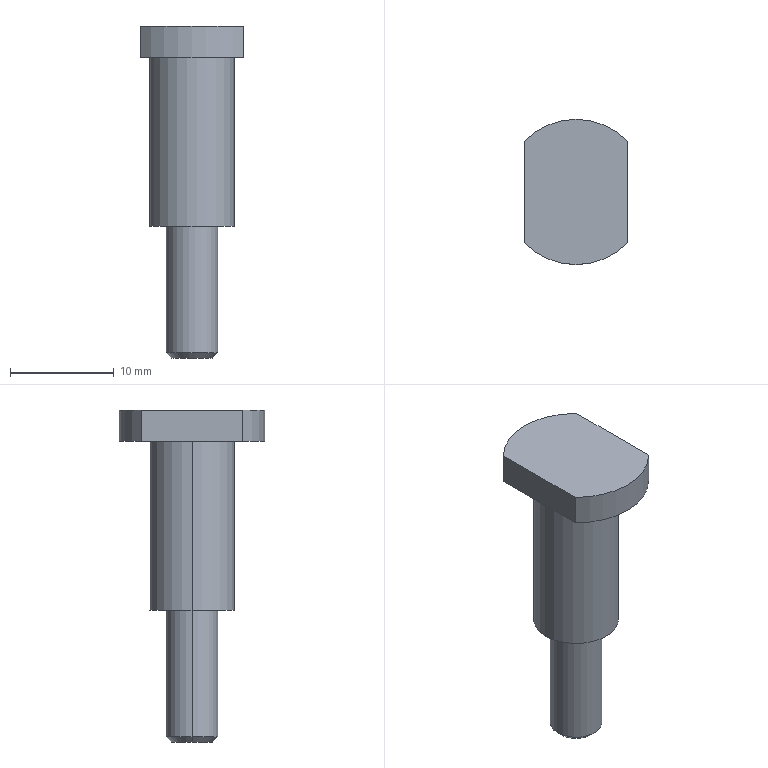Part | STEP file | 8XS900010 | 1 solid | 14 faces | box 10 x 14 x 32 mm | volume 1489 mm3 | cylinder 6 | plane 6 | cone 2 | commonest cylinder face diameters 5 x2 8.2 x2 14 x2
STEP:
#1=CARTESIAN_POINT('',(0.,0.,0.));
#2=DIRECTION('',(0.,0.,1.));
#3=DIRECTION('',(1.,0.,0.));
#4=AXIS2_PLACEMENT_3D('',#1,#2,#3);
#5=CARTESIAN_POINT('',(-2.,0.,-29.));
#6=VERTEX_POINT('',#5);
#7=CARTESIAN_POINT('',(2.,0.,-29.));
#8=VERTEX_POINT('',#7);
#9=CARTESIAN_POINT('',(0.,0.,-29.));
#10=DIRECTION('',(0.,0.,-1.));
#11=DIRECTION('',(-1.,0.,0.));
#12=AXIS2_PLACEMENT_3D('',#9,#10,#11);
#13=CIRCLE('',#12,2.);
#14=CARTESIAN_POINT('',(0.,0.,-29.));
#15=DIRECTION('',(0.,0.,1.));
#16=DIRECTION('',(1.,0.,0.));
#17=AXIS2_PLACEMENT_3D('',#14,#15,#16);
#18=CONICAL_SURFACE('',#17,2.,0.7854);
#19=CARTESIAN_POINT('',(3.142,0.));
#20=DIRECTION('',(-1.,0.));
#21=VECTOR('',#20,1.);
#22=LINE('',#19,#21);
#23=(GEOMETRIC_REPRESENTATION_CONTEXT(2)PARAMETRIC_REPRESENTATION_CONTEXT()REPRESENTATION_CONTEXT('',''));
#24=DEFINITIONAL_REPRESENTATION('',(#22),#23);
#25=PCURVE('',#18,#24);
#26=CARTESIAN_POINT('',(0.,0.,-29.));
#27=DIRECTION('',(0.,0.,-1.));
#28=DIRECTION('',(-1.,0.,0.));
#29=AXIS2_PLACEMENT_3D('',#26,#27,#28);
#30=PLANE('',#29);
#31=CARTESIAN_POINT('',(0.,0.));
#32=DIRECTION('',(1.,0.));
#33=AXIS2_PLACEMENT_2D('',#31,#32);
#34=CIRCLE('',#33,2.);
#35=(GEOMETRIC_REPRESENTATION_CONTEXT(2)PARAMETRIC_REPRESENTATION_CONTEXT()REPRESENTATION_CONTEXT('',''));
#36=DEFINITIONAL_REPRESENTATION('',(#34),#35);
#37=PCURVE('',#30,#36);
#38=SURFACE_CURVE('',#13,(#25,#37),.PCURVE_S1.);
#39=EDGE_CURVE('',#6,#8,#38,.T.);
#40=ORIENTED_EDGE('',*,*,#39,.F.);
#41=CARTESIAN_POINT('',(-2.5,0.,-28.5));
#42=VERTEX_POINT('',#41);
#43=CARTESIAN_POINT('',(-2.,0.,-29.));
#44=DIRECTION('',(-0.7071,0.,0.7071));
#45=VECTOR('',#44,1.);
#46=LINE('',#43,#45);
#47=CARTESIAN_POINT('',(3.142,0.));
#48=DIRECTION('',(0.,1.));
#49=VECTOR('',#48,1.);
#50=LINE('',#47,#49);
#51=(GEOMETRIC_REPRESENTATION_CONTEXT(2)PARAMETRIC_REPRESENTATION_CONTEXT()REPRESENTATION_CONTEXT('',''));
#52=DEFINITIONAL_REPRESENTATION('',(#50),#51);
#53=PCURVE('',#18,#52);
#54=CARTESIAN_POINT('',(0.,0.,-29.));
#55=DIRECTION('',(0.,0.,1.));
#56=DIRECTION('',(1.,0.,0.));
#57=AXIS2_PLACEMENT_3D('',#54,#55,#56);
#58=CONICAL_SURFACE('',#57,2.,0.7854);
#59=CARTESIAN_POINT('',(3.142,0.));
#60=DIRECTION('',(0.,1.));
#61=VECTOR('',#60,1.);
#62=LINE('',#59,#61);
#63=(GEOMETRIC_REPRESENTATION_CONTEXT(2)PARAMETRIC_REPRESENTATION_CONTEXT()REPRESENTATION_CONTEXT('',''));
#64=DEFINITIONAL_REPRESENTATION('',(#62),#63);
#65=PCURVE('',#58,#64);
#66=SURFACE_CURVE('',#46,(#53,#65),.PCURVE_S1.);
#67=EDGE_CURVE('',#6,#42,#66,.T.);
#68=ORIENTED_EDGE('',*,*,#67,.T.);
#69=CARTESIAN_POINT('',(2.5,0.,-28.5));
#70=VERTEX_POINT('',#69);
#71=CARTESIAN_POINT('',(0.,0.,-28.5));
#72=DIRECTION('',(0.,0.,1.));
#73=DIRECTION('',(-1.,0.,0.));
#74=AXIS2_PLACEMENT_3D('',#71,#72,#73);
#75=CIRCLE('',#74,2.5);
#76=CARTESIAN_POINT('',(-3.142,0.5));
#77=DIRECTION('',(1.,0.));
#78=VECTOR('',#77,1.);
#79=LINE('',#76,#78);
#80=(GEOMETRIC_REPRESENTATION_CONTEXT(2)PARAMETRIC_REPRESENTATION_CONTEXT()REPRESENTATION_CONTEXT('',''));
#81=DEFINITIONAL_REPRESENTATION('',(#79),#80);
#82=PCURVE('',#18,#81);
#83=CARTESIAN_POINT('',(0.,0.,-29.));
#84=DIRECTION('',(0.,0.,1.));
#85=DIRECTION('',(1.,0.,0.));
#86=AXIS2_PLACEMENT_3D('',#83,#84,#85);
#87=CYLINDRICAL_SURFACE('',#86,2.5);
#88=CARTESIAN_POINT('',(-3.142,0.5));
#89=DIRECTION('',(1.,0.));
#90=VECTOR('',#89,1.);
#91=LINE('',#88,#90);
#92=(GEOMETRIC_REPRESENTATION_CONTEXT(2)PARAMETRIC_REPRESENTATION_CONTEXT()REPRESENTATION_CONTEXT('',''));
#93=DEFINITIONAL_REPRESENTATION('',(#91),#92);
#94=PCURVE('',#87,#93);
#95=SURFACE_CURVE('',#75,(#82,#94),.PCURVE_S1.);
#96=EDGE_CURVE('',#70,#42,#95,.T.);
#97=ORIENTED_EDGE('',*,*,#96,.F.);
#98=CARTESIAN_POINT('',(2.,0.,-29.));
#99=DIRECTION('',(0.7071,0.,0.7071));
#100=VECTOR('',#99,1.);
#101=LINE('',#98,#100);
#102=CARTESIAN_POINT('',(0.,0.));
#103=DIRECTION('',(0.,1.));
#104=VECTOR('',#103,1.);
#105=LINE('',#102,#104);
#106=(GEOMETRIC_REPRESENTATION_CONTEXT(2)PARAMETRIC_REPRESENTATION_CONTEXT()REPRESENTATION_CONTEXT('',''));
#107=DEFINITIONAL_REPRESENTATION('',(#105),#106);
#108=PCURVE('',#18,#107);
#109=CARTESIAN_POINT('',(6.283,0.));
#110=DIRECTION('',(0.,1.));
#111=VECTOR('',#110,1.);
#112=LINE('',#109,#111);
#113=(GEOMETRIC_REPRESENTATION_CONTEXT(2)PARAMETRIC_REPRESENTATION_CONTEXT()REPRESENTATION_CONTEXT('',''));
#114=DEFINITIONAL_REPRESENTATION('',(#112),#113);
#115=PCURVE('',#58,#114);
#116=SURFACE_CURVE('',#101,(#108,#115),.PCURVE_S1.);
#117=EDGE_CURVE('',#8,#70,#116,.T.);
#118=ORIENTED_EDGE('',*,*,#117,.F.);
#119=EDGE_LOOP('',(#40,#68,#97,#118));
#120=FACE_BOUND('',#119,.T.);
#121=ADVANCED_FACE('',(#120),#18,.T.);
#122=ORIENTED_EDGE('',*,*,#96,.T.);
#123=CARTESIAN_POINT('',(-2.5,0.,-16.3));
#124=VERTEX_POINT('',#123);
#125=CARTESIAN_POINT('',(-2.5,0.,-29.));
#126=DIRECTION('',(0.,0.,1.));
#127=VECTOR('',#126,1.);
#128=LINE('',#125,#127);
#129=CARTESIAN_POINT('',(3.142,0.));
#130=DIRECTION('',(0.,1.));
#131=VECTOR('',#130,1.);
#132=LINE('',#129,#131);
#133=(GEOMETRIC_REPRESENTATION_CONTEXT(2)PARAMETRIC_REPRESENTATION_CONTEXT()REPRESENTATION_CONTEXT('',''));
#134=DEFINITIONAL_REPRESENTATION('',(#132),#133);
#135=PCURVE('',#87,#134);
#136=CARTESIAN_POINT('',(0.,0.,-29.));
#137=DIRECTION('',(0.,0.,1.));
#138=DIRECTION('',(1.,0.,0.));
#139=AXIS2_PLACEMENT_3D('',#136,#137,#138);
#140=CYLINDRICAL_SURFACE('',#139,2.5);
#141=CARTESIAN_POINT('',(3.142,0.));
#142=DIRECTION('',(0.,1.));
#143=VECTOR('',#142,1.);
#144=LINE('',#141,#143);
#145=(GEOMETRIC_REPRESENTATION_CONTEXT(2)PARAMETRIC_REPRESENTATION_CONTEXT()REPRESENTATION_CONTEXT('',''));
#146=DEFINITIONAL_REPRESENTATION('',(#144),#145);
#147=PCURVE('',#140,#146);
#148=SURFACE_CURVE('',#128,(#135,#147),.PCURVE_S1.);
#149=EDGE_CURVE('',#42,#124,#148,.T.);
#150=ORIENTED_EDGE('',*,*,#149,.T.);
#151=CARTESIAN_POINT('',(2.5,0.,-16.3));
#152=VERTEX_POINT('',#151);
#153=CARTESIAN_POINT('',(0.,0.,-16.3));
#154=DIRECTION('',(0.,0.,-1.));
#155=DIRECTION('',(-1.,0.,0.));
#156=AXIS2_PLACEMENT_3D('',#153,#154,#155);
#157=CIRCLE('',#156,2.5);
#158=CARTESIAN_POINT('',(3.142,12.7));
#159=DIRECTION('',(-1.,0.));
#160=VECTOR('',#159,1.);
#161=LINE('',#158,#160);
#162=(GEOMETRIC_REPRESENTATION_CONTEXT(2)PARAMETRIC_REPRESENTATION_CONTEXT()REPRESENTATION_CONTEXT('',''));
#163=DEFINITIONAL_REPRESENTATION('',(#161),#162);
#164=PCURVE('',#87,#163);
#165=CARTESIAN_POINT('',(0.,0.,-16.3));
#166=DIRECTION('',(0.,0.,-1.));
#167=DIRECTION('',(-1.,0.,0.));
#168=AXIS2_PLACEMENT_3D('',#165,#166,#167);
#169=PLANE('',#168);
#170=CARTESIAN_POINT('',(0.,0.));
#171=DIRECTION('',(1.,0.));
#172=AXIS2_PLACEMENT_2D('',#170,#171);
#173=CIRCLE('',#172,2.5);
#174=(GEOMETRIC_REPRESENTATION_CONTEXT(2)PARAMETRIC_REPRESENTATION_CONTEXT()REPRESENTATION_CONTEXT('',''));
#175=DEFINITIONAL_REPRESENTATION('',(#173),#174);
#176=PCURVE('',#169,#175);
#177=SURFACE_CURVE('',#157,(#164,#176),.PCURVE_S1.);
#178=EDGE_CURVE('',#124,#152,#177,.T.);
#179=ORIENTED_EDGE('',*,*,#178,.T.);
#180=CARTESIAN_POINT('',(2.5,0.,-29.));
#181=DIRECTION('',(0.,0.,1.));
#182=VECTOR('',#181,1.);
#183=LINE('',#180,#182);
#184=CARTESIAN_POINT('',(0.,0.));
#185=DIRECTION('',(0.,1.));
#186=VECTOR('',#185,1.);
#187=LINE('',#184,#186);
#188=(GEOMETRIC_REPRESENTATION_CONTEXT(2)PARAMETRIC_REPRESENTATION_CONTEXT()REPRESENTATION_CONTEXT('',''));
#189=DEFINITIONAL_REPRESENTATION('',(#187),#188);
#190=PCURVE('',#87,#189);
#191=CARTESIAN_POINT('',(6.283,0.));
#192=DIRECTION('',(0.,1.));
#193=VECTOR('',#192,1.);
#194=LINE('',#191,#193);
#195=(GEOMETRIC_REPRESENTATION_CONTEXT(2)PARAMETRIC_REPRESENTATION_CONTEXT()REPRESENTATION_CONTEXT('',''));
#196=DEFINITIONAL_REPRESENTATION('',(#194),#195);
#197=PCURVE('',#140,#196);
#198=SURFACE_CURVE('',#183,(#190,#197),.PCURVE_S1.);
#199=EDGE_CURVE('',#70,#152,#198,.T.);
#200=ORIENTED_EDGE('',*,*,#199,.F.);
#201=EDGE_LOOP('',(#122,#150,#179,#200));
#202=FACE_BOUND('',#201,.T.);
#203=ADVANCED_FACE('',(#202),#87,.T.);
#204=CARTESIAN_POINT('',(-4.1,0.,-16.3));
#205=VERTEX_POINT('',#204);
#206=CARTESIAN_POINT('',(4.1,0.,-16.3));
#207=VERTEX_POINT('',#206);
#208=CARTESIAN_POINT('',(0.,0.,-16.3));
#209=DIRECTION('',(0.,0.,-1.));
#210=DIRECTION('',(-1.,0.,0.));
#211=AXIS2_PLACEMENT_3D('',#208,#209,#210);
#212=CIRCLE('',#211,4.1);
#213=CARTESIAN_POINT('',(0.,0.,-16.3));
#214=DIRECTION('',(0.,0.,1.));
#215=DIRECTION('',(1.,0.,0.));
#216=AXIS2_PLACEMENT_3D('',#213,#214,#215);
#217=CYLINDRICAL_SURFACE('',#216,4.1);
#218=CARTESIAN_POINT('',(3.142,0.));
#219=DIRECTION('',(-1.,0.));
#220=VECTOR('',#219,1.);
#221=LINE('',#218,#220);
#222=(GEOMETRIC_REPRESENTATION_CONTEXT(2)PARAMETRIC_REPRESENTATION_CONTEXT()REPRESENTATION_CONTEXT('',''));
#223=DEFINITIONAL_REPRESENTATION('',(#221),#222);
#224=PCURVE('',#217,#223);
#225=CARTESIAN_POINT('',(0.,0.));
#226=DIRECTION('',(1.,0.));
#227=AXIS2_PLACEMENT_2D('',#225,#226);
#228=CIRCLE('',#227,4.1);
#229=(GEOMETRIC_REPRESENTATION_CONTEXT(2)PARAMETRIC_REPRESENTATION_CONTEXT()REPRESENTATION_CONTEXT('',''));
#230=DEFINITIONAL_REPRESENTATION('',(#228),#229);
#231=PCURVE('',#169,#230);
#232=SURFACE_CURVE('',#212,(#224,#231),.PCURVE_S1.);
#233=EDGE_CURVE('',#205,#207,#232,.T.);
#234=ORIENTED_EDGE('',*,*,#233,.F.);
#235=CARTESIAN_POINT('',(-4.1,0.,0.));
#236=VERTEX_POINT('',#235);
#237=CARTESIAN_POINT('',(-4.1,0.,-16.3));
#238=DIRECTION('',(0.,0.,1.));
#239=VECTOR('',#238,1.);
#240=LINE('',#237,#239);
#241=CARTESIAN_POINT('',(3.142,0.));
#242=DIRECTION('',(0.,1.));
#243=VECTOR('',#242,1.);
#244=LINE('',#241,#243);
#245=(GEOMETRIC_REPRESENTATION_CONTEXT(2)PARAMETRIC_REPRESENTATION_CONTEXT()REPRESENTATION_CONTEXT('',''));
#246=DEFINITIONAL_REPRESENTATION('',(#244),#245);
#247=PCURVE('',#217,#246);
#248=CARTESIAN_POINT('',(0.,0.,-16.3));
#249=DIRECTION('',(0.,0.,1.));
#250=DIRECTION('',(1.,0.,0.));
#251=AXIS2_PLACEMENT_3D('',#248,#249,#250);
#252=CYLINDRICAL_SURFACE('',#251,4.1);
#253=CARTESIAN_POINT('',(3.142,0.));
#254=DIRECTION('',(0.,1.));
#255=VECTOR('',#254,1.);
#256=LINE('',#253,#255);
#257=(GEOMETRIC_REPRESENTATION_CONTEXT(2)PARAMETRIC_REPRESENTATION_CONTEXT()REPRESENTATION_CONTEXT('',''));
#258=DEFINITIONAL_REPRESENTATION('',(#256),#257);
#259=PCURVE('',#252,#258);
#260=SURFACE_CURVE('',#240,(#247,#259),.PCURVE_S1.);
#261=EDGE_CURVE('',#205,#236,#260,.T.);
#262=ORIENTED_EDGE('',*,*,#261,.T.);
#263=CARTESIAN_POINT('',(4.1,0.,0.));
#264=VERTEX_POINT('',#263);
#265=CARTESIAN_POINT('',(0.,0.,0.));
#266=DIRECTION('',(0.,0.,-1.));
#267=DIRECTION('',(1.,0.,0.));
#268=AXIS2_PLACEMENT_3D('',#265,#266,#267);
#269=CIRCLE('',#268,4.1);
#270=CARTESIAN_POINT('',(6.283,16.3));
#271=DIRECTION('',(-1.,0.));
#272=VECTOR('',#271,1.);
#273=LINE('',#270,#272);
#274=(GEOMETRIC_REPRESENTATION_CONTEXT(2)PARAMETRIC_REPRESENTATION_CONTEXT()REPRESENTATION_CONTEXT('',''));
#275=DEFINITIONAL_REPRESENTATION('',(#273),#274);
#276=PCURVE('',#217,#275);
#277=CARTESIAN_POINT('',(0.,0.,0.));
#278=DIRECTION('',(0.,0.,1.));
#279=DIRECTION('',(1.,0.,0.));
#280=AXIS2_PLACEMENT_3D('',#277,#278,#279);
#281=PLANE('',#280);
#282=CARTESIAN_POINT('',(4.1,0.));
#283=CARTESIAN_POINT('',(4.1,-7.101));
#284=CARTESIAN_POINT('',(-2.05,-3.551));
#285=CARTESIAN_POINT('',(-8.2,0.));
#286=CARTESIAN_POINT('',(-2.05,3.551));
#287=CARTESIAN_POINT('',(4.1,7.101));
#288=CARTESIAN_POINT('',(4.1,0.));
#289=(BOUNDED_CURVE()B_SPLINE_CURVE(2,(#282,#283,#284,#285,#286,#287,#288),.UNSPECIFIED.,.T.,.F.)B_SPLINE_CURVE_WITH_KNOTS((1,2,2,2,2,1),(-2.094,0.,2.094,4.189,6.283,8.378),.UNSPECIFIED.)CURVE()GEOMETRIC_REPRESENTATION_ITEM()RATIONAL_B_SPLINE_CURVE((1.,0.5,1.,0.5,1.,0.5,1.))REPRESENTATION_ITEM(''));
#290=(GEOMETRIC_REPRESENTATION_CONTEXT(2)PARAMETRIC_REPRESENTATION_CONTEXT()REPRESENTATION_CONTEXT('',''));
#291=DEFINITIONAL_REPRESENTATION('',(#289),#290);
#292=PCURVE('',#281,#291);
#293=SURFACE_CURVE('',#269,(#276,#292),.PCURVE_S1.);
#294=EDGE_CURVE('',#236,#264,#293,.T.);
#295=ORIENTED_EDGE('',*,*,#294,.T.);
#296=CARTESIAN_POINT('',(4.1,0.,-16.3));
#297=DIRECTION('',(0.,0.,1.));
#298=VECTOR('',#297,1.);
#299=LINE('',#296,#298);
#300=CARTESIAN_POINT('',(0.,0.));
#301=DIRECTION('',(0.,1.));
#302=VECTOR('',#301,1.);
#303=LINE('',#300,#302);
#304=(GEOMETRIC_REPRESENTATION_CONTEXT(2)PARAMETRIC_REPRESENTATION_CONTEXT()REPRESENTATION_CONTEXT('',''));
#305=DEFINITIONAL_REPRESENTATION('',(#303),#304);
#306=PCURVE('',#217,#305);
#307=CARTESIAN_POINT('',(6.283,0.));
#308=DIRECTION('',(0.,1.));
#309=VECTOR('',#308,1.);
#310=LINE('',#307,#309);
#311=(GEOMETRIC_REPRESENTATION_CONTEXT(2)PARAMETRIC_REPRESENTATION_CONTEXT()REPRESENTATION_CONTEXT('',''));
#312=DEFINITIONAL_REPRESENTATION('',(#310),#311);
#313=PCURVE('',#252,#312);
#314=SURFACE_CURVE('',#299,(#306,#313),.PCURVE_S1.);
#315=EDGE_CURVE('',#207,#264,#314,.T.);
#316=ORIENTED_EDGE('',*,*,#315,.F.);
#317=EDGE_LOOP('',(#234,#262,#295,#316));
#318=FACE_BOUND('',#317,.T.);
#319=ADVANCED_FACE('',(#318),#217,.T.);
#320=CARTESIAN_POINT('',(0.,0.,-16.3));
#321=DIRECTION('',(0.,0.,-1.));
#322=DIRECTION('',(-1.,0.,0.));
#323=AXIS2_PLACEMENT_3D('',#320,#321,#322);
#324=CIRCLE('',#323,4.1);
#325=CARTESIAN_POINT('',(0.,0.));
#326=DIRECTION('',(1.,0.));
#327=AXIS2_PLACEMENT_2D('',#325,#326);
#328=CIRCLE('',#327,4.1);
#329=(GEOMETRIC_REPRESENTATION_CONTEXT(2)PARAMETRIC_REPRESENTATION_CONTEXT()REPRESENTATION_CONTEXT('',''));
#330=DEFINITIONAL_REPRESENTATION('',(#328),#329);
#331=PCURVE('',#169,#330);
#332=CARTESIAN_POINT('',(9.425,0.));
#333=DIRECTION('',(-1.,0.));
#334=VECTOR('',#333,1.);
#335=LINE('',#332,#334);
#336=(GEOMETRIC_REPRESENTATION_CONTEXT(2)PARAMETRIC_REPRESENTATION_CONTEXT()REPRESENTATION_CONTEXT('',''));
#337=DEFINITIONAL_REPRESENTATION('',(#335),#336);
#338=PCURVE('',#252,#337);
#339=SURFACE_CURVE('',#324,(#331,#338),.PCURVE_S1.);
#340=EDGE_CURVE('',#207,#205,#339,.T.);
#341=ORIENTED_EDGE('',*,*,#340,.T.);
#342=ORIENTED_EDGE('',*,*,#233,.T.);
#343=EDGE_LOOP('',(#341,#342));
#344=FACE_BOUND('',#343,.T.);
#345=CARTESIAN_POINT('',(0.,0.,-16.3));
#346=DIRECTION('',(0.,0.,-1.));
#347=DIRECTION('',(-1.,0.,0.));
#348=AXIS2_PLACEMENT_3D('',#345,#346,#347);
#349=CIRCLE('',#348,2.5);
#350=CARTESIAN_POINT('',(0.,0.));
#351=DIRECTION('',(1.,0.));
#352=AXIS2_PLACEMENT_2D('',#350,#351);
#353=CIRCLE('',#352,2.5);
#354=(GEOMETRIC_REPRESENTATION_CONTEXT(2)PARAMETRIC_REPRESENTATION_CONTEXT()REPRESENTATION_CONTEXT('',''));
#355=DEFINITIONAL_REPRESENTATION('',(#353),#354);
#356=PCURVE('',#169,#355);
#357=CARTESIAN_POINT('',(9.425,12.7));
#358=DIRECTION('',(-1.,0.));
#359=VECTOR('',#358,1.);
#360=LINE('',#357,#359);
#361=(GEOMETRIC_REPRESENTATION_CONTEXT(2)PARAMETRIC_REPRESENTATION_CONTEXT()REPRESENTATION_CONTEXT('',''));
#362=DEFINITIONAL_REPRESENTATION('',(#360),#361);
#363=PCURVE('',#140,#362);
#364=SURFACE_CURVE('',#349,(#356,#363),.PCURVE_S1.);
#365=EDGE_CURVE('',#152,#124,#364,.T.);
#366=ORIENTED_EDGE('',*,*,#365,.F.);
#367=ORIENTED_EDGE('',*,*,#178,.F.);
#368=EDGE_LOOP('',(#366,#367));
#369=FACE_BOUND('',#368,.T.);
#370=ADVANCED_FACE('',(#344,#369),#169,.T.);
#371=CARTESIAN_POINT('',(5.,4.899,0.));
#372=VERTEX_POINT('',#371);
#373=CARTESIAN_POINT('',(-5.,4.899,0.));
#374=VERTEX_POINT('',#373);
#375=CARTESIAN_POINT('',(0.,0.,0.));
#376=DIRECTION('',(0.,0.,1.));
#377=DIRECTION('',(1.,0.,0.));
#378=AXIS2_PLACEMENT_3D('',#375,#376,#377);
#379=CIRCLE('',#378,7.);
#380=CARTESIAN_POINT('',(0.,0.));
#381=DIRECTION('',(1.,0.));
#382=AXIS2_PLACEMENT_2D('',#380,#381);
#383=CIRCLE('',#382,7.);
#384=(GEOMETRIC_REPRESENTATION_CONTEXT(2)PARAMETRIC_REPRESENTATION_CONTEXT()REPRESENTATION_CONTEXT('',''));
#385=DEFINITIONAL_REPRESENTATION('',(#383),#384);
#386=PCURVE('',#281,#385);
#387=CARTESIAN_POINT('',(0.,0.,3.));
#388=DIRECTION('',(0.,0.,-1.));
#389=DIRECTION('',(-1.,0.,0.));
#390=AXIS2_PLACEMENT_3D('',#387,#388,#389);
#391=CYLINDRICAL_SURFACE('',#390,7.);
#392=CARTESIAN_POINT('',(3.142,3.));
#393=DIRECTION('',(-1.,0.));
#394=VECTOR('',#393,1.);
#395=LINE('',#392,#394);
#396=(GEOMETRIC_REPRESENTATION_CONTEXT(2)PARAMETRIC_REPRESENTATION_CONTEXT()REPRESENTATION_CONTEXT('',''));
#397=DEFINITIONAL_REPRESENTATION('',(#395),#396);
#398=PCURVE('',#391,#397);
#399=SURFACE_CURVE('',#379,(#386,#398),.PCURVE_S1.);
#400=EDGE_CURVE('',#372,#374,#399,.T.);
#401=ORIENTED_EDGE('',*,*,#400,.F.);
#402=CARTESIAN_POINT('',(5.,-4.899,0.));
#403=VERTEX_POINT('',#402);
#404=CARTESIAN_POINT('',(5.,4.899,0.));
#405=DIRECTION('',(0.,1.,0.));
#406=VECTOR('',#405,1.);
#407=LINE('',#404,#406);
#408=CARTESIAN_POINT('',(5.,4.899));
#409=DIRECTION('',(0.,1.));
#410=VECTOR('',#409,1.);
#411=LINE('',#408,#410);
#412=(GEOMETRIC_REPRESENTATION_CONTEXT(2)PARAMETRIC_REPRESENTATION_CONTEXT()REPRESENTATION_CONTEXT('',''));
#413=DEFINITIONAL_REPRESENTATION('',(#411),#412);
#414=PCURVE('',#281,#413);
#415=CARTESIAN_POINT('',(5.,4.899,3.));
#416=DIRECTION('',(-1.,0.,0.));
#417=DIRECTION('',(0.,0.,1.));
#418=AXIS2_PLACEMENT_3D('',#415,#416,#417);
#419=PLANE('',#418);
#420=CARTESIAN_POINT('',(-3.,0.));
#421=DIRECTION('',(0.,1.));
#422=VECTOR('',#421,1.);
#423=LINE('',#420,#422);
#424=(GEOMETRIC_REPRESENTATION_CONTEXT(2)PARAMETRIC_REPRESENTATION_CONTEXT()REPRESENTATION_CONTEXT('',''));
#425=DEFINITIONAL_REPRESENTATION('',(#423),#424);
#426=PCURVE('',#419,#425);
#427=SURFACE_CURVE('',#407,(#414,#426),.PCURVE_S1.);
#428=EDGE_CURVE('',#403,#372,#427,.T.);
#429=ORIENTED_EDGE('',*,*,#428,.F.);
#430=CARTESIAN_POINT('',(-5.,-4.899,0.));
#431=VERTEX_POINT('',#430);
#432=CARTESIAN_POINT('',(0.,0.,0.));
#433=DIRECTION('',(0.,0.,1.));
#434=DIRECTION('',(1.,0.,0.));
#435=AXIS2_PLACEMENT_3D('',#432,#433,#434);
#436=CIRCLE('',#435,7.);
#437=CARTESIAN_POINT('',(0.,0.));
#438=DIRECTION('',(1.,0.));
#439=AXIS2_PLACEMENT_2D('',#437,#438);
#440=CIRCLE('',#439,7.);
#441=(GEOMETRIC_REPRESENTATION_CONTEXT(2)PARAMETRIC_REPRESENTATION_CONTEXT()REPRESENTATION_CONTEXT('',''));
#442=DEFINITIONAL_REPRESENTATION('',(#440),#441);
#443=PCURVE('',#281,#442);
#444=CARTESIAN_POINT('',(0.,0.,3.));
#445=DIRECTION('',(0.,0.,-1.));
#446=DIRECTION('',(-1.,0.,0.));
#447=AXIS2_PLACEMENT_3D('',#444,#445,#446);
#448=CYLINDRICAL_SURFACE('',#447,7.);
#449=CARTESIAN_POINT('',(9.425,3.));
#450=DIRECTION('',(-1.,0.));
#451=VECTOR('',#450,1.);
#452=LINE('',#449,#451);
#453=(GEOMETRIC_REPRESENTATION_CONTEXT(2)PARAMETRIC_REPRESENTATION_CONTEXT()REPRESENTATION_CONTEXT('',''));
#454=DEFINITIONAL_REPRESENTATION('',(#452),#453);
#455=PCURVE('',#448,#454);
#456=SURFACE_CURVE('',#436,(#443,#455),.PCURVE_S1.);
#457=EDGE_CURVE('',#431,#403,#456,.T.);
#458=ORIENTED_EDGE('',*,*,#457,.F.);
#459=CARTESIAN_POINT('',(-5.,4.899,0.));
#460=DIRECTION('',(0.,-1.,0.));
#461=VECTOR('',#460,1.);
#462=LINE('',#459,#461);
#463=CARTESIAN_POINT('',(-5.,4.899));
#464=DIRECTION('',(0.,-1.));
#465=VECTOR('',#464,1.);
#466=LINE('',#463,#465);
#467=(GEOMETRIC_REPRESENTATION_CONTEXT(2)PARAMETRIC_REPRESENTATION_CONTEXT()REPRESENTATION_CONTEXT('',''));
#468=DEFINITIONAL_REPRESENTATION('',(#466),#467);
#469=PCURVE('',#281,#468);
#470=CARTESIAN_POINT('',(-5.,4.899,3.));
#471=DIRECTION('',(1.,0.,0.));
#472=DIRECTION('',(0.,0.,-1.));
#473=AXIS2_PLACEMENT_3D('',#470,#471,#472);
#474=PLANE('',#473);
#475=CARTESIAN_POINT('',(3.,0.));
#476=DIRECTION('',(0.,-1.));
#477=VECTOR('',#476,1.);
#478=LINE('',#475,#477);
#479=(GEOMETRIC_REPRESENTATION_CONTEXT(2)PARAMETRIC_REPRESENTATION_CONTEXT()REPRESENTATION_CONTEXT('',''));
#480=DEFINITIONAL_REPRESENTATION('',(#478),#479);
#481=PCURVE('',#474,#480);
#482=SURFACE_CURVE('',#462,(#469,#481),.PCURVE_S1.);
#483=EDGE_CURVE('',#374,#431,#482,.T.);
#484=ORIENTED_EDGE('',*,*,#483,.F.);
#485=EDGE_LOOP('',(#401,#429,#458,#484));
#486=FACE_BOUND('',#485,.T.);
#487=CARTESIAN_POINT('',(0.,0.,0.));
#488=DIRECTION('',(0.,0.,-1.));
#489=DIRECTION('',(1.,0.,0.));
#490=AXIS2_PLACEMENT_3D('',#487,#488,#489);
#491=CIRCLE('',#490,4.1);
#492=CARTESIAN_POINT('',(4.1,0.));
#493=CARTESIAN_POINT('',(4.1,-7.101));
#494=CARTESIAN_POINT('',(-2.05,-3.551));
#495=CARTESIAN_POINT('',(-8.2,0.));
#496=CARTESIAN_POINT('',(-2.05,3.551));
#497=CARTESIAN_POINT('',(4.1,7.101));
#498=CARTESIAN_POINT('',(4.1,0.));
#499=(BOUNDED_CURVE()B_SPLINE_CURVE(2,(#492,#493,#494,#495,#496,#497,#498),.UNSPECIFIED.,.T.,.F.)B_SPLINE_CURVE_WITH_KNOTS((1,2,2,2,2,1),(-2.094,0.,2.094,4.189,6.283,8.378),.UNSPECIFIED.)CURVE()GEOMETRIC_REPRESENTATION_ITEM()RATIONAL_B_SPLINE_CURVE((1.,0.5,1.,0.5,1.,0.5,1.))REPRESENTATION_ITEM(''));
#500=(GEOMETRIC_REPRESENTATION_CONTEXT(2)PARAMETRIC_REPRESENTATION_CONTEXT()REPRESENTATION_CONTEXT('',''));
#501=DEFINITIONAL_REPRESENTATION('',(#499),#500);
#502=PCURVE('',#281,#501);
#503=CARTESIAN_POINT('',(6.283,16.3));
#504=DIRECTION('',(-1.,0.));
#505=VECTOR('',#504,1.);
#506=LINE('',#503,#505);
#507=(GEOMETRIC_REPRESENTATION_CONTEXT(2)PARAMETRIC_REPRESENTATION_CONTEXT()REPRESENTATION_CONTEXT('',''));
#508=DEFINITIONAL_REPRESENTATION('',(#506),#507);
#509=PCURVE('',#252,#508);
#510=SURFACE_CURVE('',#491,(#502,#509),.PCURVE_S1.);
#511=EDGE_CURVE('',#264,#236,#510,.T.);
#512=ORIENTED_EDGE('',*,*,#511,.F.);
#513=ORIENTED_EDGE('',*,*,#294,.F.);
#514=EDGE_LOOP('',(#512,#513));
#515=FACE_BOUND('',#514,.T.);
#516=ADVANCED_FACE('',(#486,#515),#281,.F.);
#517=ORIENTED_EDGE('',*,*,#400,.T.);
#518=CARTESIAN_POINT('',(-5.,4.899,3.));
#519=VERTEX_POINT('',#518);
#520=CARTESIAN_POINT('',(-5.,4.899,3.));
#521=DIRECTION('',(0.,0.,-1.));
#522=VECTOR('',#521,1.);
#523=LINE('',#520,#522);
#524=CARTESIAN_POINT('',(0.7752,0.));
#525=DIRECTION('',(0.,1.));
#526=VECTOR('',#525,1.);
#527=LINE('',#524,#526);
#528=(GEOMETRIC_REPRESENTATION_CONTEXT(2)PARAMETRIC_REPRESENTATION_CONTEXT()REPRESENTATION_CONTEXT('',''));
#529=DEFINITIONAL_REPRESENTATION('',(#527),#528);
#530=PCURVE('',#391,#529);
#531=CARTESIAN_POINT('',(0.,0.));
#532=DIRECTION('',(1.,0.));
#533=VECTOR('',#532,1.);
#534=LINE('',#531,#533);
#535=(GEOMETRIC_REPRESENTATION_CONTEXT(2)PARAMETRIC_REPRESENTATION_CONTEXT()REPRESENTATION_CONTEXT('',''));
#536=DEFINITIONAL_REPRESENTATION('',(#534),#535);
#537=PCURVE('',#474,#536);
#538=SURFACE_CURVE('',#523,(#530,#537),.PCURVE_S1.);
#539=EDGE_CURVE('',#519,#374,#538,.T.);
#540=ORIENTED_EDGE('',*,*,#539,.F.);
#541=CARTESIAN_POINT('',(5.,4.899,3.));
#542=VERTEX_POINT('',#541);
#543=CARTESIAN_POINT('',(0.,0.,3.));
#544=DIRECTION('',(0.,0.,1.));
#545=DIRECTION('',(1.,0.,0.));
#546=AXIS2_PLACEMENT_3D('',#543,#544,#545);
#547=CIRCLE('',#546,7.);
#548=CARTESIAN_POINT('',(3.142,0.));
#549=DIRECTION('',(-1.,0.));
#550=VECTOR('',#549,1.);
#551=LINE('',#548,#550);
#552=(GEOMETRIC_REPRESENTATION_CONTEXT(2)PARAMETRIC_REPRESENTATION_CONTEXT()REPRESENTATION_CONTEXT('',''));
#553=DEFINITIONAL_REPRESENTATION('',(#551),#552);
#554=PCURVE('',#391,#553);
#555=CARTESIAN_POINT('',(0.,0.,3.));
#556=DIRECTION('',(0.,0.,1.));
#557=DIRECTION('',(1.,0.,0.));
#558=AXIS2_PLACEMENT_3D('',#555,#556,#557);
#559=PLANE('',#558);
#560=CARTESIAN_POINT('',(0.,0.));
#561=DIRECTION('',(1.,0.));
#562=AXIS2_PLACEMENT_2D('',#560,#561);
#563=CIRCLE('',#562,7.);
#564=(GEOMETRIC_REPRESENTATION_CONTEXT(2)PARAMETRIC_REPRESENTATION_CONTEXT()REPRESENTATION_CONTEXT('',''));
#565=DEFINITIONAL_REPRESENTATION('',(#563),#564);
#566=PCURVE('',#559,#565);
#567=SURFACE_CURVE('',#547,(#554,#566),.PCURVE_S1.);
#568=EDGE_CURVE('',#542,#519,#567,.T.);
#569=ORIENTED_EDGE('',*,*,#568,.F.);
#570=CARTESIAN_POINT('',(5.,4.899,3.));
#571=DIRECTION('',(0.,0.,-1.));
#572=VECTOR('',#571,1.);
#573=LINE('',#570,#572);
#574=CARTESIAN_POINT('',(2.366,0.));
#575=DIRECTION('',(0.,1.));
#576=VECTOR('',#575,1.);
#577=LINE('',#574,#576);
#578=(GEOMETRIC_REPRESENTATION_CONTEXT(2)PARAMETRIC_REPRESENTATION_CONTEXT()REPRESENTATION_CONTEXT('',''));
#579=DEFINITIONAL_REPRESENTATION('',(#577),#578);
#580=PCURVE('',#391,#579);
#581=CARTESIAN_POINT('',(0.,0.));
#582=DIRECTION('',(-1.,0.));
#583=VECTOR('',#582,1.);
#584=LINE('',#581,#583);
#585=(GEOMETRIC_REPRESENTATION_CONTEXT(2)PARAMETRIC_REPRESENTATION_CONTEXT()REPRESENTATION_CONTEXT('',''));
#586=DEFINITIONAL_REPRESENTATION('',(#584),#585);
#587=PCURVE('',#419,#586);
#588=SURFACE_CURVE('',#573,(#580,#587),.PCURVE_S1.);
#589=EDGE_CURVE('',#542,#372,#588,.T.);
#590=ORIENTED_EDGE('',*,*,#589,.T.);
#591=EDGE_LOOP('',(#517,#540,#569,#590));
#592=FACE_BOUND('',#591,.T.);
#593=ADVANCED_FACE('',(#592),#391,.T.);
#594=ORIENTED_EDGE('',*,*,#483,.T.);
#595=CARTESIAN_POINT('',(-5.,-4.899,3.));
#596=VERTEX_POINT('',#595);
#597=CARTESIAN_POINT('',(-5.,-4.899,3.));
#598=DIRECTION('',(0.,0.,-1.));
#599=VECTOR('',#598,1.);
#600=LINE('',#597,#599);
#601=CARTESIAN_POINT('',(0.,-9.798));
#602=DIRECTION('',(1.,0.));
#603=VECTOR('',#602,1.);
#604=LINE('',#601,#603);
#605=(GEOMETRIC_REPRESENTATION_CONTEXT(2)PARAMETRIC_REPRESENTATION_CONTEXT()REPRESENTATION_CONTEXT('',''));
#606=DEFINITIONAL_REPRESENTATION('',(#604),#605);
#607=PCURVE('',#474,#606);
#608=CARTESIAN_POINT('',(5.508,0.));
#609=DIRECTION('',(0.,1.));
#610=VECTOR('',#609,1.);
#611=LINE('',#608,#610);
#612=(GEOMETRIC_REPRESENTATION_CONTEXT(2)PARAMETRIC_REPRESENTATION_CONTEXT()REPRESENTATION_CONTEXT('',''));
#613=DEFINITIONAL_REPRESENTATION('',(#611),#612);
#614=PCURVE('',#448,#613);
#615=SURFACE_CURVE('',#600,(#607,#614),.PCURVE_S1.);
#616=EDGE_CURVE('',#596,#431,#615,.T.);
#617=ORIENTED_EDGE('',*,*,#616,.F.);
#618=CARTESIAN_POINT('',(-5.,4.899,3.));
#619=DIRECTION('',(0.,-1.,0.));
#620=VECTOR('',#619,1.);
#621=LINE('',#618,#620);
#622=CARTESIAN_POINT('',(0.,0.));
#623=DIRECTION('',(0.,-1.));
#624=VECTOR('',#623,1.);
#625=LINE('',#622,#624);
#626=(GEOMETRIC_REPRESENTATION_CONTEXT(2)PARAMETRIC_REPRESENTATION_CONTEXT()REPRESENTATION_CONTEXT('',''));
#627=DEFINITIONAL_REPRESENTATION('',(#625),#626);
#628=PCURVE('',#474,#627);
#629=CARTESIAN_POINT('',(-5.,4.899));
#630=DIRECTION('',(0.,-1.));
#631=VECTOR('',#630,1.);
#632=LINE('',#629,#631);
#633=(GEOMETRIC_REPRESENTATION_CONTEXT(2)PARAMETRIC_REPRESENTATION_CONTEXT()REPRESENTATION_CONTEXT('',''));
#634=DEFINITIONAL_REPRESENTATION('',(#632),#633);
#635=PCURVE('',#559,#634);
#636=SURFACE_CURVE('',#621,(#628,#635),.PCURVE_S1.);
#637=EDGE_CURVE('',#519,#596,#636,.T.);
#638=ORIENTED_EDGE('',*,*,#637,.F.);
#639=ORIENTED_EDGE('',*,*,#539,.T.);
#640=EDGE_LOOP('',(#594,#617,#638,#639));
#641=FACE_BOUND('',#640,.T.);
#642=ADVANCED_FACE('',(#641),#474,.F.);
#643=ORIENTED_EDGE('',*,*,#457,.T.);
#644=CARTESIAN_POINT('',(5.,-4.899,3.));
#645=VERTEX_POINT('',#644);
#646=CARTESIAN_POINT('',(5.,-4.899,3.));
#647=DIRECTION('',(0.,0.,-1.));
#648=VECTOR('',#647,1.);
#649=LINE('',#646,#648);
#650=CARTESIAN_POINT('',(3.917,0.));
#651=DIRECTION('',(0.,1.));
#652=VECTOR('',#651,1.);
#653=LINE('',#650,#652);
#654=(GEOMETRIC_REPRESENTATION_CONTEXT(2)PARAMETRIC_REPRESENTATION_CONTEXT()REPRESENTATION_CONTEXT('',''));
#655=DEFINITIONAL_REPRESENTATION('',(#653),#654);
#656=PCURVE('',#448,#655);
#657=CARTESIAN_POINT('',(0.,-9.798));
#658=DIRECTION('',(-1.,0.));
#659=VECTOR('',#658,1.);
#660=LINE('',#657,#659);
#661=(GEOMETRIC_REPRESENTATION_CONTEXT(2)PARAMETRIC_REPRESENTATION_CONTEXT()REPRESENTATION_CONTEXT('',''));
#662=DEFINITIONAL_REPRESENTATION('',(#660),#661);
#663=PCURVE('',#419,#662);
#664=SURFACE_CURVE('',#649,(#656,#663),.PCURVE_S1.);
#665=EDGE_CURVE('',#645,#403,#664,.T.);
#666=ORIENTED_EDGE('',*,*,#665,.F.);
#667=CARTESIAN_POINT('',(0.,0.,3.));
#668=DIRECTION('',(0.,0.,1.));
#669=DIRECTION('',(1.,0.,0.));
#670=AXIS2_PLACEMENT_3D('',#667,#668,#669);
#671=CIRCLE('',#670,7.);
#672=CARTESIAN_POINT('',(9.425,0.));
#673=DIRECTION('',(-1.,0.));
#674=VECTOR('',#673,1.);
#675=LINE('',#672,#674);
#676=(GEOMETRIC_REPRESENTATION_CONTEXT(2)PARAMETRIC_REPRESENTATION_CONTEXT()REPRESENTATION_CONTEXT('',''));
#677=DEFINITIONAL_REPRESENTATION('',(#675),#676);
#678=PCURVE('',#448,#677);
#679=CARTESIAN_POINT('',(0.,0.));
#680=DIRECTION('',(1.,0.));
#681=AXIS2_PLACEMENT_2D('',#679,#680);
#682=CIRCLE('',#681,7.);
#683=(GEOMETRIC_REPRESENTATION_CONTEXT(2)PARAMETRIC_REPRESENTATION_CONTEXT()REPRESENTATION_CONTEXT('',''));
#684=DEFINITIONAL_REPRESENTATION('',(#682),#683);
#685=PCURVE('',#559,#684);
#686=SURFACE_CURVE('',#671,(#678,#685),.PCURVE_S1.);
#687=EDGE_CURVE('',#596,#645,#686,.T.);
#688=ORIENTED_EDGE('',*,*,#687,.F.);
#689=ORIENTED_EDGE('',*,*,#616,.T.);
#690=EDGE_LOOP('',(#643,#666,#688,#689));
#691=FACE_BOUND('',#690,.T.);
#692=ADVANCED_FACE('',(#691),#448,.T.);
#693=ORIENTED_EDGE('',*,*,#428,.T.);
#694=ORIENTED_EDGE('',*,*,#589,.F.);
#695=CARTESIAN_POINT('',(5.,4.899,3.));
#696=DIRECTION('',(0.,1.,0.));
#697=VECTOR('',#696,1.);
#698=LINE('',#695,#697);
#699=CARTESIAN_POINT('',(0.,0.));
#700=DIRECTION('',(0.,1.));
#701=VECTOR('',#700,1.);
#702=LINE('',#699,#701);
#703=(GEOMETRIC_REPRESENTATION_CONTEXT(2)PARAMETRIC_REPRESENTATION_CONTEXT()REPRESENTATION_CONTEXT('',''));
#704=DEFINITIONAL_REPRESENTATION('',(#702),#703);
#705=PCURVE('',#419,#704);
#706=CARTESIAN_POINT('',(5.,4.899));
#707=DIRECTION('',(0.,1.));
#708=VECTOR('',#707,1.);
#709=LINE('',#706,#708);
#710=(GEOMETRIC_REPRESENTATION_CONTEXT(2)PARAMETRIC_REPRESENTATION_CONTEXT()REPRESENTATION_CONTEXT('',''));
#711=DEFINITIONAL_REPRESENTATION('',(#709),#710);
#712=PCURVE('',#559,#711);
#713=SURFACE_CURVE('',#698,(#705,#712),.PCURVE_S1.);
#714=EDGE_CURVE('',#645,#542,#713,.T.);
#715=ORIENTED_EDGE('',*,*,#714,.F.);
#716=ORIENTED_EDGE('',*,*,#665,.T.);
#717=EDGE_LOOP('',(#693,#694,#715,#716));
#718=FACE_BOUND('',#717,.T.);
#719=ADVANCED_FACE('',(#718),#419,.F.);
#720=ORIENTED_EDGE('',*,*,#568,.T.);
#721=ORIENTED_EDGE('',*,*,#637,.T.);
#722=ORIENTED_EDGE('',*,*,#687,.T.);
#723=ORIENTED_EDGE('',*,*,#714,.T.);
#724=EDGE_LOOP('',(#720,#721,#722,#723));
#725=FACE_BOUND('',#724,.T.);
#726=ADVANCED_FACE('',(#725),#559,.T.);
#727=ORIENTED_EDGE('',*,*,#261,.F.);
#728=ORIENTED_EDGE('',*,*,#340,.F.);
#729=ORIENTED_EDGE('',*,*,#315,.T.);
#730=ORIENTED_EDGE('',*,*,#511,.T.);
#731=EDGE_LOOP('',(#727,#728,#729,#730));
#732=FACE_BOUND('',#731,.T.);
#733=ADVANCED_FACE('',(#732),#252,.T.);
#734=ORIENTED_EDGE('',*,*,#149,.F.);
#735=CARTESIAN_POINT('',(0.,0.,-28.5));
#736=DIRECTION('',(0.,0.,1.));
#737=DIRECTION('',(-1.,0.,0.));
#738=AXIS2_PLACEMENT_3D('',#735,#736,#737);
#739=CIRCLE('',#738,2.5);
#740=CARTESIAN_POINT('',(3.142,0.5));
#741=DIRECTION('',(1.,0.));
#742=VECTOR('',#741,1.);
#743=LINE('',#740,#742);
#744=(GEOMETRIC_REPRESENTATION_CONTEXT(2)PARAMETRIC_REPRESENTATION_CONTEXT()REPRESENTATION_CONTEXT('',''));
#745=DEFINITIONAL_REPRESENTATION('',(#743),#744);
#746=PCURVE('',#140,#745);
#747=CARTESIAN_POINT('',(3.142,0.5));
#748=DIRECTION('',(1.,0.));
#749=VECTOR('',#748,1.);
#750=LINE('',#747,#749);
#751=(GEOMETRIC_REPRESENTATION_CONTEXT(2)PARAMETRIC_REPRESENTATION_CONTEXT()REPRESENTATION_CONTEXT('',''));
#752=DEFINITIONAL_REPRESENTATION('',(#750),#751);
#753=PCURVE('',#58,#752);
#754=SURFACE_CURVE('',#739,(#746,#753),.PCURVE_S1.);
#755=EDGE_CURVE('',#42,#70,#754,.T.);
#756=ORIENTED_EDGE('',*,*,#755,.T.);
#757=ORIENTED_EDGE('',*,*,#199,.T.);
#758=ORIENTED_EDGE('',*,*,#365,.T.);
#759=EDGE_LOOP('',(#734,#756,#757,#758));
#760=FACE_BOUND('',#759,.T.);
#761=ADVANCED_FACE('',(#760),#140,.T.);
#762=CARTESIAN_POINT('',(0.,0.,-29.));
#763=DIRECTION('',(0.,0.,-1.));
#764=DIRECTION('',(-1.,0.,0.));
#765=AXIS2_PLACEMENT_3D('',#762,#763,#764);
#766=CIRCLE('',#765,2.);
#767=CARTESIAN_POINT('',(0.,0.));
#768=DIRECTION('',(1.,0.));
#769=AXIS2_PLACEMENT_2D('',#767,#768);
#770=CIRCLE('',#769,2.);
#771=(GEOMETRIC_REPRESENTATION_CONTEXT(2)PARAMETRIC_REPRESENTATION_CONTEXT()REPRESENTATION_CONTEXT('',''));
#772=DEFINITIONAL_REPRESENTATION('',(#770),#771);
#773=PCURVE('',#30,#772);
#774=CARTESIAN_POINT('',(9.425,0.));
#775=DIRECTION('',(-1.,0.));
#776=VECTOR('',#775,1.);
#777=LINE('',#774,#776);
#778=(GEOMETRIC_REPRESENTATION_CONTEXT(2)PARAMETRIC_REPRESENTATION_CONTEXT()REPRESENTATION_CONTEXT('',''));
#779=DEFINITIONAL_REPRESENTATION('',(#777),#778);
#780=PCURVE('',#58,#779);
#781=SURFACE_CURVE('',#766,(#773,#780),.PCURVE_S1.);
#782=EDGE_CURVE('',#8,#6,#781,.T.);
#783=ORIENTED_EDGE('',*,*,#782,.T.);
#784=ORIENTED_EDGE('',*,*,#39,.T.);
#785=EDGE_LOOP('',(#783,#784));
#786=FACE_BOUND('',#785,.T.);
#787=ADVANCED_FACE('',(#786),#30,.T.);
#788=ORIENTED_EDGE('',*,*,#67,.F.);
#789=ORIENTED_EDGE('',*,*,#782,.F.);
#790=ORIENTED_EDGE('',*,*,#117,.T.);
#791=ORIENTED_EDGE('',*,*,#755,.F.);
#792=EDGE_LOOP('',(#788,#789,#790,#791));
#793=FACE_BOUND('',#792,.T.);
#794=ADVANCED_FACE('',(#793),#58,.T.);
#795=CLOSED_SHELL('',(#121,#203,#319,#370,#516,#593,#642,#692,#719,#726,#733,#761,#787,#794));
#796=MANIFOLD_SOLID_BREP('',#795);
#797=(LENGTH_UNIT()NAMED_UNIT(*)SI_UNIT(.MILLI.,.METRE.));
#798=UNCERTAINTY_MEASURE_WITH_UNIT(LENGTH_MEASURE(0.0000001),#797,'','');
#799=(NAMED_UNIT(*)PLANE_ANGLE_UNIT()SI_UNIT($,.RADIAN.));
#800=(NAMED_UNIT(*)SI_UNIT($,.STERADIAN.)SOLID_ANGLE_UNIT());
#801=(GEOMETRIC_REPRESENTATION_CONTEXT(3)GLOBAL_UNCERTAINTY_ASSIGNED_CONTEXT((#798))GLOBAL_UNIT_ASSIGNED_CONTEXT((#797,#799,#800))REPRESENTATION_CONTEXT('',''));
#802=ADVANCED_BREP_SHAPE_REPRESENTATION('',(#4,#796),#801);